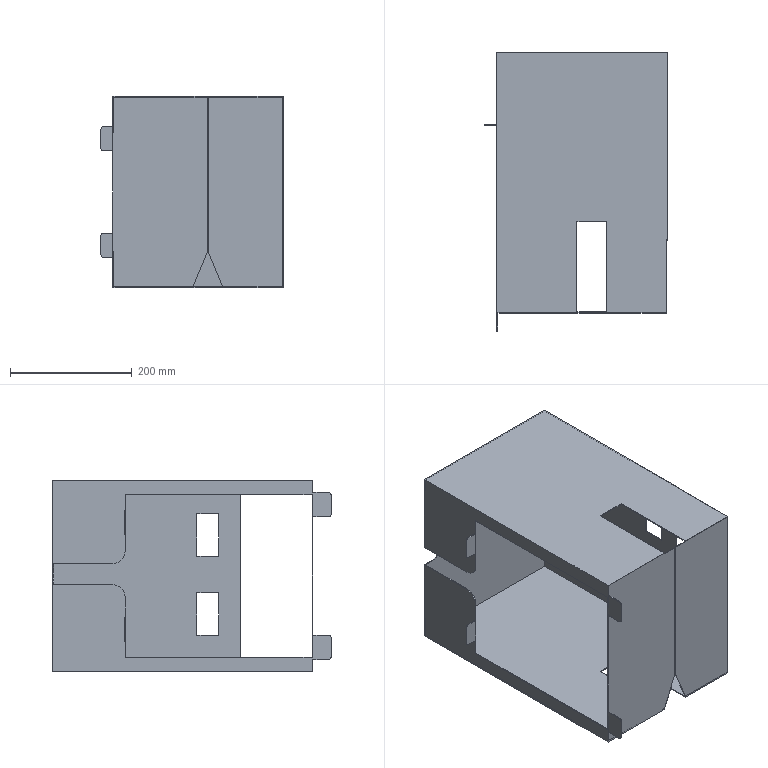Part | STEP file | cover 10 | 1 solid | 70 faces | box 300 x 458 x 315 mm | volume 804947 mm3 | plane 59 | cylinder 11 | commonest cylinder face diameters 10 x8 40 x2 35 x1